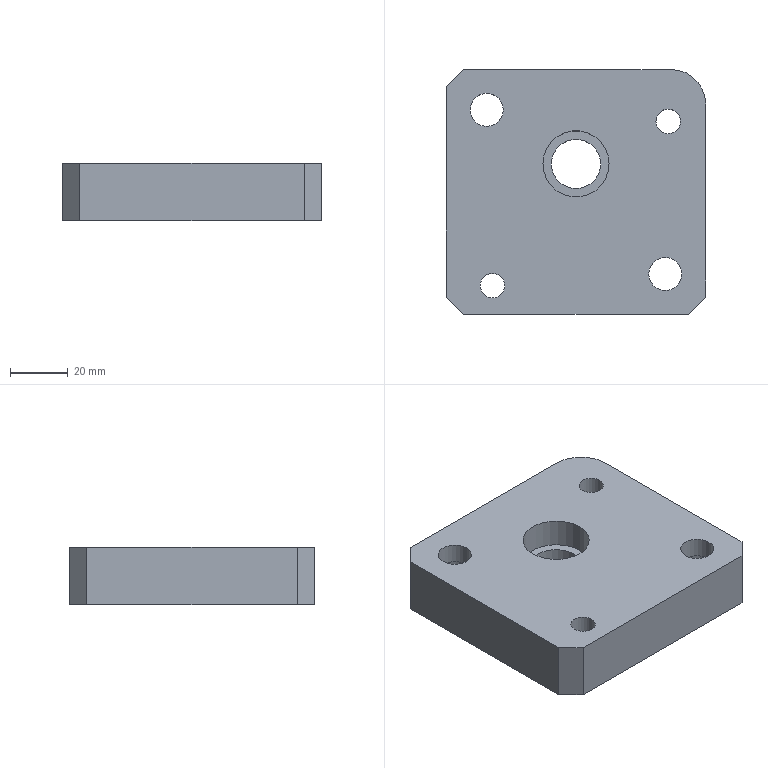Part | STEP file | lll_id3138_x_t | 1 solid | 21 faces | box 90 x 85 x 20 mm | volume 134500 mm3 | plane 12 | cylinder 9 | commonest cylinder face diameters 8.505 x2 11.509 x2 18.007 x2 17.1 x1 23 x1 24 x1
STEP:
#1=CARTESIAN_POINT('',(403.747,257.75,2.5));
#2=VERTEX_POINT('',#1);
#3=CARTESIAN_POINT('',(408.,257.75,2.5));
#4=DIRECTION('',(0.,0.,-1.));
#5=DIRECTION('',(-1.,0.,0.));
#6=AXIS2_PLACEMENT_3D('',#3,#4,#5);
#7=CIRCLE('',#6,4.253);
#8=EDGE_CURVE('',#2,#2,#7,.T.);
#9=ORIENTED_EDGE('',*,*,#8,.F.);
#10=EDGE_LOOP('',(#9));
#11=FACE_BOUND('',#10,.T.);
#12=CARTESIAN_POINT('',(415.003,318.75,2.5));
#13=VERTEX_POINT('',#12);
#14=CARTESIAN_POINT('',(406.,318.75,2.5));
#15=DIRECTION('',(0.,0.,1.));
#16=DIRECTION('',(1.,0.,0.));
#17=AXIS2_PLACEMENT_3D('',#14,#15,#16);
#18=CIRCLE('',#17,9.004);
#19=EDGE_CURVE('',#13,#13,#18,.T.);
#20=ORIENTED_EDGE('',*,*,#19,.T.);
#21=EDGE_LOOP('',(#20));
#22=FACE_BOUND('',#21,.T.);
#23=CARTESIAN_POINT('',(464.747,314.75,2.5));
#24=VERTEX_POINT('',#23);
#25=CARTESIAN_POINT('',(469.,314.75,2.5));
#26=DIRECTION('',(0.,0.,-1.));
#27=DIRECTION('',(-1.,0.,0.));
#28=AXIS2_PLACEMENT_3D('',#25,#26,#27);
#29=CIRCLE('',#28,4.253);
#30=EDGE_CURVE('',#24,#24,#29,.T.);
#31=ORIENTED_EDGE('',*,*,#30,.F.);
#32=EDGE_LOOP('',(#31));
#33=FACE_BOUND('',#32,.T.);
#34=CARTESIAN_POINT('',(470.,332.75,2.5));
#35=VERTEX_POINT('',#34);
#36=CARTESIAN_POINT('',(398.,332.75,2.5));
#37=VERTEX_POINT('',#36);
#38=CARTESIAN_POINT('',(437.,332.75,2.5));
#39=DIRECTION('',(-1.,0.,0.));
#40=VECTOR('',#39,1.);
#41=LINE('',#38,#40);
#42=EDGE_CURVE('',#35,#37,#41,.T.);
#43=ORIENTED_EDGE('',*,*,#42,.F.);
#44=CARTESIAN_POINT('',(482.,320.75,2.5));
#45=VERTEX_POINT('',#44);
#46=CARTESIAN_POINT('',(470.,320.75,2.5));
#47=DIRECTION('',(0.,0.,-1.));
#48=DIRECTION('',(-1.,0.,0.));
#49=AXIS2_PLACEMENT_3D('',#46,#47,#48);
#50=CIRCLE('',#49,12.);
#51=EDGE_CURVE('',#35,#45,#50,.T.);
#52=ORIENTED_EDGE('',*,*,#51,.T.);
#53=CARTESIAN_POINT('',(482.,253.75,2.5));
#54=VERTEX_POINT('',#53);
#55=CARTESIAN_POINT('',(482.,291.75,2.5));
#56=DIRECTION('',(0.,1.,0.));
#57=VECTOR('',#56,1.);
#58=LINE('',#55,#57);
#59=EDGE_CURVE('',#54,#45,#58,.T.);
#60=ORIENTED_EDGE('',*,*,#59,.F.);
#61=CARTESIAN_POINT('',(476.,247.75,2.5));
#62=VERTEX_POINT('',#61);
#63=CARTESIAN_POINT('',(478.5,250.25,2.5));
#64=DIRECTION('',(-0.7071,-0.7071,0.));
#65=VECTOR('',#64,1.);
#66=LINE('',#63,#65);
#67=EDGE_CURVE('',#54,#62,#66,.T.);
#68=ORIENTED_EDGE('',*,*,#67,.T.);
#69=CARTESIAN_POINT('',(398.,247.75,2.5));
#70=VERTEX_POINT('',#69);
#71=CARTESIAN_POINT('',(437.,247.75,2.5));
#72=DIRECTION('',(1.,0.,0.));
#73=VECTOR('',#72,1.);
#74=LINE('',#71,#73);
#75=EDGE_CURVE('',#70,#62,#74,.T.);
#76=ORIENTED_EDGE('',*,*,#75,.F.);
#77=CARTESIAN_POINT('',(392.,253.75,2.5));
#78=VERTEX_POINT('',#77);
#79=CARTESIAN_POINT('',(395.5,250.25,2.5));
#80=DIRECTION('',(-0.7071,0.7071,0.));
#81=VECTOR('',#80,1.);
#82=LINE('',#79,#81);
#83=EDGE_CURVE('',#70,#78,#82,.T.);
#84=ORIENTED_EDGE('',*,*,#83,.T.);
#85=CARTESIAN_POINT('',(392.,326.75,2.5));
#86=VERTEX_POINT('',#85);
#87=CARTESIAN_POINT('',(392.,291.75,2.5));
#88=DIRECTION('',(0.,-1.,0.));
#89=VECTOR('',#88,1.);
#90=LINE('',#87,#89);
#91=EDGE_CURVE('',#86,#78,#90,.T.);
#92=ORIENTED_EDGE('',*,*,#91,.F.);
#93=CARTESIAN_POINT('',(397.,331.75,2.5));
#94=DIRECTION('',(0.7071,0.7071,0.));
#95=VECTOR('',#94,1.);
#96=LINE('',#93,#95);
#97=EDGE_CURVE('',#86,#37,#96,.T.);
#98=ORIENTED_EDGE('',*,*,#97,.T.);
#99=EDGE_LOOP('',(#43,#52,#60,#68,#76,#84,#92,#98));
#100=FACE_BOUND('',#99,.T.);
#101=CARTESIAN_POINT('',(428.45,300.,2.5));
#102=VERTEX_POINT('',#101);
#103=CARTESIAN_POINT('',(437.,300.,2.5));
#104=DIRECTION('',(0.,0.,1.));
#105=DIRECTION('',(-1.,0.,0.));
#106=AXIS2_PLACEMENT_3D('',#103,#104,#105);
#107=CIRCLE('',#106,8.55);
#108=EDGE_CURVE('',#102,#102,#107,.T.);
#109=ORIENTED_EDGE('',*,*,#108,.T.);
#110=EDGE_LOOP('',(#109));
#111=FACE_BOUND('',#110,.T.);
#112=CARTESIAN_POINT('',(477.003,261.75,2.5));
#113=VERTEX_POINT('',#112);
#114=CARTESIAN_POINT('',(468.,261.75,2.5));
#115=DIRECTION('',(0.,0.,1.));
#116=DIRECTION('',(1.,0.,0.));
#117=AXIS2_PLACEMENT_3D('',#114,#115,#116);
#118=CIRCLE('',#117,9.004);
#119=EDGE_CURVE('',#113,#113,#118,.T.);
#120=ORIENTED_EDGE('',*,*,#119,.T.);
#121=EDGE_LOOP('',(#120));
#122=FACE_BOUND('',#121,.T.);
#123=CARTESIAN_POINT('',(437.,291.75,2.5));
#124=DIRECTION('',(0.,0.,-1.));
#125=DIRECTION('',(1.,0.,0.));
#126=AXIS2_PLACEMENT_3D('',#123,#124,#125);
#127=PLANE('',#126);
#128=ADVANCED_FACE('',(#11,#22,#33,#100,#111,#122),#127,.T.);
#129=CARTESIAN_POINT('',(412.252,257.75,22.5));
#130=VERTEX_POINT('',#129);
#131=CARTESIAN_POINT('',(408.,257.75,22.5));
#132=DIRECTION('',(0.,0.,1.));
#133=DIRECTION('',(1.,0.,0.));
#134=AXIS2_PLACEMENT_3D('',#131,#132,#133);
#135=CIRCLE('',#134,4.253);
#136=EDGE_CURVE('',#130,#130,#135,.T.);
#137=ORIENTED_EDGE('',*,*,#136,.F.);
#138=EDGE_LOOP('',(#137));
#139=FACE_BOUND('',#138,.T.);
#140=CARTESIAN_POINT('',(473.754,261.75,22.5));
#141=VERTEX_POINT('',#140);
#142=CARTESIAN_POINT('',(468.,261.75,22.5));
#143=DIRECTION('',(0.,0.,1.));
#144=DIRECTION('',(1.,0.,0.));
#145=AXIS2_PLACEMENT_3D('',#142,#143,#144);
#146=CIRCLE('',#145,5.755);
#147=EDGE_CURVE('',#141,#141,#146,.T.);
#148=ORIENTED_EDGE('',*,*,#147,.F.);
#149=EDGE_LOOP('',(#148));
#150=FACE_BOUND('',#149,.T.);
#151=CARTESIAN_POINT('',(411.754,318.75,22.5));
#152=VERTEX_POINT('',#151);
#153=CARTESIAN_POINT('',(406.,318.75,22.5));
#154=DIRECTION('',(0.,0.,1.));
#155=DIRECTION('',(1.,0.,0.));
#156=AXIS2_PLACEMENT_3D('',#153,#154,#155);
#157=CIRCLE('',#156,5.755);
#158=EDGE_CURVE('',#152,#152,#157,.T.);
#159=ORIENTED_EDGE('',*,*,#158,.F.);
#160=EDGE_LOOP('',(#159));
#161=FACE_BOUND('',#160,.T.);
#162=CARTESIAN_POINT('',(473.252,314.75,22.5));
#163=VERTEX_POINT('',#162);
#164=CARTESIAN_POINT('',(469.,314.75,22.5));
#165=DIRECTION('',(0.,0.,1.));
#166=DIRECTION('',(1.,0.,0.));
#167=AXIS2_PLACEMENT_3D('',#164,#165,#166);
#168=CIRCLE('',#167,4.253);
#169=EDGE_CURVE('',#163,#163,#168,.T.);
#170=ORIENTED_EDGE('',*,*,#169,.F.);
#171=EDGE_LOOP('',(#170));
#172=FACE_BOUND('',#171,.T.);
#173=CARTESIAN_POINT('',(482.,320.75,22.5));
#174=VERTEX_POINT('',#173);
#175=CARTESIAN_POINT('',(482.,253.75,22.5));
#176=VERTEX_POINT('',#175);
#177=CARTESIAN_POINT('',(482.,291.75,22.5));
#178=DIRECTION('',(0.,-1.,0.));
#179=VECTOR('',#178,1.);
#180=LINE('',#177,#179);
#181=EDGE_CURVE('',#174,#176,#180,.T.);
#182=ORIENTED_EDGE('',*,*,#181,.F.);
#183=CARTESIAN_POINT('',(470.,332.75,22.5));
#184=VERTEX_POINT('',#183);
#185=CARTESIAN_POINT('',(470.,320.75,22.5));
#186=DIRECTION('',(0.,0.,1.));
#187=DIRECTION('',(1.,0.,0.));
#188=AXIS2_PLACEMENT_3D('',#185,#186,#187);
#189=CIRCLE('',#188,12.);
#190=EDGE_CURVE('',#174,#184,#189,.T.);
#191=ORIENTED_EDGE('',*,*,#190,.T.);
#192=CARTESIAN_POINT('',(398.,332.75,22.5));
#193=VERTEX_POINT('',#192);
#194=CARTESIAN_POINT('',(437.,332.75,22.5));
#195=DIRECTION('',(1.,0.,0.));
#196=VECTOR('',#195,1.);
#197=LINE('',#194,#196);
#198=EDGE_CURVE('',#193,#184,#197,.T.);
#199=ORIENTED_EDGE('',*,*,#198,.F.);
#200=CARTESIAN_POINT('',(392.,326.75,22.5));
#201=VERTEX_POINT('',#200);
#202=CARTESIAN_POINT('',(397.,331.75,22.5));
#203=DIRECTION('',(-0.7071,-0.7071,0.));
#204=VECTOR('',#203,1.);
#205=LINE('',#202,#204);
#206=EDGE_CURVE('',#193,#201,#205,.T.);
#207=ORIENTED_EDGE('',*,*,#206,.T.);
#208=CARTESIAN_POINT('',(392.,253.75,22.5));
#209=VERTEX_POINT('',#208);
#210=CARTESIAN_POINT('',(392.,291.75,22.5));
#211=DIRECTION('',(0.,1.,0.));
#212=VECTOR('',#211,1.);
#213=LINE('',#210,#212);
#214=EDGE_CURVE('',#209,#201,#213,.T.);
#215=ORIENTED_EDGE('',*,*,#214,.F.);
#216=CARTESIAN_POINT('',(398.,247.75,22.5));
#217=VERTEX_POINT('',#216);
#218=CARTESIAN_POINT('',(395.5,250.25,22.5));
#219=DIRECTION('',(0.7071,-0.7071,0.));
#220=VECTOR('',#219,1.);
#221=LINE('',#218,#220);
#222=EDGE_CURVE('',#209,#217,#221,.T.);
#223=ORIENTED_EDGE('',*,*,#222,.T.);
#224=CARTESIAN_POINT('',(476.,247.75,22.5));
#225=VERTEX_POINT('',#224);
#226=CARTESIAN_POINT('',(437.,247.75,22.5));
#227=DIRECTION('',(-1.,0.,0.));
#228=VECTOR('',#227,1.);
#229=LINE('',#226,#228);
#230=EDGE_CURVE('',#225,#217,#229,.T.);
#231=ORIENTED_EDGE('',*,*,#230,.F.);
#232=CARTESIAN_POINT('',(478.5,250.25,22.5));
#233=DIRECTION('',(0.7071,0.7071,0.));
#234=VECTOR('',#233,1.);
#235=LINE('',#232,#234);
#236=EDGE_CURVE('',#225,#176,#235,.T.);
#237=ORIENTED_EDGE('',*,*,#236,.T.);
#238=EDGE_LOOP('',(#182,#191,#199,#207,#215,#223,#231,#237));
#239=FACE_BOUND('',#238,.T.);
#240=CARTESIAN_POINT('',(448.5,300.,22.5));
#241=VERTEX_POINT('',#240);
#242=CARTESIAN_POINT('',(437.,300.,22.5));
#243=DIRECTION('',(0.,0.,-1.));
#244=DIRECTION('',(1.,0.,0.));
#245=AXIS2_PLACEMENT_3D('',#242,#243,#244);
#246=CIRCLE('',#245,11.5);
#247=EDGE_CURVE('',#241,#241,#246,.T.);
#248=ORIENTED_EDGE('',*,*,#247,.T.);
#249=EDGE_LOOP('',(#248));
#250=FACE_BOUND('',#249,.T.);
#251=CARTESIAN_POINT('',(437.,291.75,22.5));
#252=DIRECTION('',(0.,0.,1.));
#253=DIRECTION('',(-1.,0.,0.));
#254=AXIS2_PLACEMENT_3D('',#251,#252,#253);
#255=PLANE('',#254);
#256=ADVANCED_FACE('',(#139,#150,#161,#172,#239,#250),#255,.T.);
#257=ORIENTED_EDGE('',*,*,#198,.T.);
#258=CARTESIAN_POINT('',(470.,332.75,2.5));
#259=DIRECTION('',(0.,0.,-1.));
#260=VECTOR('',#259,1.);
#261=LINE('',#258,#260);
#262=EDGE_CURVE('',#184,#35,#261,.T.);
#263=ORIENTED_EDGE('',*,*,#262,.T.);
#264=ORIENTED_EDGE('',*,*,#42,.T.);
#265=CARTESIAN_POINT('',(398.,332.75,2.5));
#266=DIRECTION('',(0.,0.,1.));
#267=VECTOR('',#266,1.);
#268=LINE('',#265,#267);
#269=EDGE_CURVE('',#37,#193,#268,.T.);
#270=ORIENTED_EDGE('',*,*,#269,.T.);
#271=EDGE_LOOP('',(#257,#263,#264,#270));
#272=FACE_OUTER_BOUND('',#271,.T.);
#273=CARTESIAN_POINT('',(437.,332.75,2.5));
#274=DIRECTION('',(0.,1.,0.));
#275=DIRECTION('',(0.,0.,-1.));
#276=AXIS2_PLACEMENT_3D('',#273,#274,#275);
#277=PLANE('',#276);
#278=ADVANCED_FACE('',(#272),#277,.T.);
#279=ORIENTED_EDGE('',*,*,#59,.T.);
#280=CARTESIAN_POINT('',(482.,320.75,2.5));
#281=DIRECTION('',(0.,0.,1.));
#282=VECTOR('',#281,1.);
#283=LINE('',#280,#282);
#284=EDGE_CURVE('',#45,#174,#283,.T.);
#285=ORIENTED_EDGE('',*,*,#284,.T.);
#286=ORIENTED_EDGE('',*,*,#181,.T.);
#287=CARTESIAN_POINT('',(482.,253.75,2.5));
#288=DIRECTION('',(0.,0.,-1.));
#289=VECTOR('',#288,1.);
#290=LINE('',#287,#289);
#291=EDGE_CURVE('',#176,#54,#290,.T.);
#292=ORIENTED_EDGE('',*,*,#291,.T.);
#293=EDGE_LOOP('',(#279,#285,#286,#292));
#294=FACE_OUTER_BOUND('',#293,.T.);
#295=CARTESIAN_POINT('',(482.,291.75,2.5));
#296=DIRECTION('',(1.,0.,0.));
#297=DIRECTION('',(0.,0.,1.));
#298=AXIS2_PLACEMENT_3D('',#295,#296,#297);
#299=PLANE('',#298);
#300=ADVANCED_FACE('',(#294),#299,.T.);
#301=ORIENTED_EDGE('',*,*,#75,.T.);
#302=CARTESIAN_POINT('',(476.,247.75,2.5));
#303=DIRECTION('',(0.,0.,1.));
#304=VECTOR('',#303,1.);
#305=LINE('',#302,#304);
#306=EDGE_CURVE('',#62,#225,#305,.T.);
#307=ORIENTED_EDGE('',*,*,#306,.T.);
#308=ORIENTED_EDGE('',*,*,#230,.T.);
#309=CARTESIAN_POINT('',(398.,247.75,2.5));
#310=DIRECTION('',(0.,0.,-1.));
#311=VECTOR('',#310,1.);
#312=LINE('',#309,#311);
#313=EDGE_CURVE('',#217,#70,#312,.T.);
#314=ORIENTED_EDGE('',*,*,#313,.T.);
#315=EDGE_LOOP('',(#301,#307,#308,#314));
#316=FACE_OUTER_BOUND('',#315,.T.);
#317=CARTESIAN_POINT('',(437.,247.75,2.5));
#318=DIRECTION('',(0.,-1.,0.));
#319=DIRECTION('',(0.,0.,1.));
#320=AXIS2_PLACEMENT_3D('',#317,#318,#319);
#321=PLANE('',#320);
#322=ADVANCED_FACE('',(#316),#321,.T.);
#323=ORIENTED_EDGE('',*,*,#214,.T.);
#324=CARTESIAN_POINT('',(392.,326.75,2.5));
#325=DIRECTION('',(0.,0.,-1.));
#326=VECTOR('',#325,1.);
#327=LINE('',#324,#326);
#328=EDGE_CURVE('',#201,#86,#327,.T.);
#329=ORIENTED_EDGE('',*,*,#328,.T.);
#330=ORIENTED_EDGE('',*,*,#91,.T.);
#331=CARTESIAN_POINT('',(392.,253.75,2.5));
#332=DIRECTION('',(0.,0.,1.));
#333=VECTOR('',#332,1.);
#334=LINE('',#331,#333);
#335=EDGE_CURVE('',#78,#209,#334,.T.);
#336=ORIENTED_EDGE('',*,*,#335,.T.);
#337=EDGE_LOOP('',(#323,#329,#330,#336));
#338=FACE_OUTER_BOUND('',#337,.T.);
#339=CARTESIAN_POINT('',(392.,291.75,2.5));
#340=DIRECTION('',(-1.,0.,0.));
#341=DIRECTION('',(0.,0.,-1.));
#342=AXIS2_PLACEMENT_3D('',#339,#340,#341);
#343=PLANE('',#342);
#344=ADVANCED_FACE('',(#338),#343,.T.);
#345=CARTESIAN_POINT('',(428.45,300.,12.5));
#346=VERTEX_POINT('',#345);
#347=CARTESIAN_POINT('',(437.,300.,12.5));
#348=DIRECTION('',(0.,0.,-1.));
#349=DIRECTION('',(-1.,0.,0.));
#350=AXIS2_PLACEMENT_3D('',#347,#348,#349);
#351=CIRCLE('',#350,8.55);
#352=EDGE_CURVE('',#346,#346,#351,.T.);
#353=ORIENTED_EDGE('',*,*,#352,.F.);
#354=EDGE_LOOP('',(#353));
#355=FACE_BOUND('',#354,.T.);
#356=ORIENTED_EDGE('',*,*,#108,.F.);
#357=EDGE_LOOP('',(#356));
#358=FACE_BOUND('',#357,.T.);
#359=CARTESIAN_POINT('',(437.,300.,125.));
#360=DIRECTION('',(0.,0.,-1.));
#361=DIRECTION('',(1.,0.,0.));
#362=AXIS2_PLACEMENT_3D('',#359,#360,#361);
#363=CYLINDRICAL_SURFACE('',#362,8.55);
#364=ADVANCED_FACE('',(#355,#358),#363,.F.);
#365=CARTESIAN_POINT('',(425.5,300.,12.5));
#366=VERTEX_POINT('',#365);
#367=CARTESIAN_POINT('',(437.,300.,12.5));
#368=DIRECTION('',(0.,0.,1.));
#369=DIRECTION('',(-1.,0.,0.));
#370=AXIS2_PLACEMENT_3D('',#367,#368,#369);
#371=CIRCLE('',#370,11.5);
#372=EDGE_CURVE('',#366,#366,#371,.T.);
#373=ORIENTED_EDGE('',*,*,#372,.F.);
#374=EDGE_LOOP('',(#373));
#375=FACE_BOUND('',#374,.T.);
#376=ORIENTED_EDGE('',*,*,#247,.F.);
#377=EDGE_LOOP('',(#376));
#378=FACE_BOUND('',#377,.T.);
#379=CARTESIAN_POINT('',(437.,300.,12.5));
#380=DIRECTION('',(0.,0.,1.));
#381=DIRECTION('',(1.,0.,0.));
#382=AXIS2_PLACEMENT_3D('',#379,#380,#381);
#383=CYLINDRICAL_SURFACE('',#382,11.5);
#384=ADVANCED_FACE('',(#375,#378),#383,.F.);
#385=ORIENTED_EDGE('',*,*,#352,.T.);
#386=EDGE_LOOP('',(#385));
#387=FACE_BOUND('',#386,.T.);
#388=ORIENTED_EDGE('',*,*,#372,.T.);
#389=EDGE_LOOP('',(#388));
#390=FACE_BOUND('',#389,.T.);
#391=CARTESIAN_POINT('',(437.,300.,12.5));
#392=DIRECTION('',(0.,0.,-1.));
#393=DIRECTION('',(-1.,0.,0.));
#394=AXIS2_PLACEMENT_3D('',#391,#392,#393);
#395=PLANE('',#394);
#396=ADVANCED_FACE('',(#387,#390),#395,.F.);
#397=ORIENTED_EDGE('',*,*,#169,.T.);
#398=EDGE_LOOP('',(#397));
#399=FACE_BOUND('',#398,.T.);
#400=ORIENTED_EDGE('',*,*,#30,.T.);
#401=EDGE_LOOP('',(#400));
#402=FACE_BOUND('',#401,.T.);
#403=CARTESIAN_POINT('',(469.,314.75,-2.5));
#404=DIRECTION('',(0.,0.,1.));
#405=DIRECTION('',(1.,0.,0.));
#406=AXIS2_PLACEMENT_3D('',#403,#404,#405);
#407=CYLINDRICAL_SURFACE('',#406,4.253);
#408=ADVANCED_FACE('',(#399,#402),#407,.F.);
#409=ORIENTED_EDGE('',*,*,#158,.T.);
#410=EDGE_LOOP('',(#409));
#411=FACE_BOUND('',#410,.T.);
#412=CARTESIAN_POINT('',(411.754,318.75,15.5));
#413=VERTEX_POINT('',#412);
#414=CARTESIAN_POINT('',(406.,318.75,15.5));
#415=DIRECTION('',(0.,0.,1.));
#416=DIRECTION('',(1.,0.,0.));
#417=AXIS2_PLACEMENT_3D('',#414,#415,#416);
#418=CIRCLE('',#417,5.755);
#419=EDGE_CURVE('',#413,#413,#418,.T.);
#420=ORIENTED_EDGE('',*,*,#419,.F.);
#421=EDGE_LOOP('',(#420));
#422=FACE_BOUND('',#421,.T.);
#423=CARTESIAN_POINT('',(406.,318.75,-2.5));
#424=DIRECTION('',(0.,0.,1.));
#425=DIRECTION('',(1.,0.,0.));
#426=AXIS2_PLACEMENT_3D('',#423,#424,#425);
#427=CYLINDRICAL_SURFACE('',#426,5.755);
#428=ADVANCED_FACE('',(#411,#422),#427,.F.);
#429=ORIENTED_EDGE('',*,*,#419,.T.);
#430=EDGE_LOOP('',(#429));
#431=FACE_BOUND('',#430,.T.);
#432=CARTESIAN_POINT('',(415.003,318.75,15.5));
#433=VERTEX_POINT('',#432);
#434=CARTESIAN_POINT('',(406.,318.75,15.5));
#435=DIRECTION('',(0.,0.,1.));
#436=DIRECTION('',(1.,0.,0.));
#437=AXIS2_PLACEMENT_3D('',#434,#435,#436);
#438=CIRCLE('',#437,9.004);
#439=EDGE_CURVE('',#433,#433,#438,.T.);
#440=ORIENTED_EDGE('',*,*,#439,.F.);
#441=EDGE_LOOP('',(#440));
#442=FACE_BOUND('',#441,.T.);
#443=CARTESIAN_POINT('',(406.,318.75,15.5));
#444=DIRECTION('',(0.,0.,1.));
#445=DIRECTION('',(1.,0.,0.));
#446=AXIS2_PLACEMENT_3D('',#443,#444,#445);
#447=PLANE('',#446);
#448=ADVANCED_FACE('',(#431,#442),#447,.F.);
#449=ORIENTED_EDGE('',*,*,#439,.T.);
#450=EDGE_LOOP('',(#449));
#451=FACE_BOUND('',#450,.T.);
#452=ORIENTED_EDGE('',*,*,#19,.F.);
#453=EDGE_LOOP('',(#452));
#454=FACE_BOUND('',#453,.T.);
#455=CARTESIAN_POINT('',(406.,318.75,2.5));
#456=DIRECTION('',(0.,0.,1.));
#457=DIRECTION('',(1.,0.,0.));
#458=AXIS2_PLACEMENT_3D('',#455,#456,#457);
#459=CYLINDRICAL_SURFACE('',#458,9.004);
#460=ADVANCED_FACE('',(#451,#454),#459,.F.);
#461=ORIENTED_EDGE('',*,*,#147,.T.);
#462=EDGE_LOOP('',(#461));
#463=FACE_BOUND('',#462,.T.);
#464=CARTESIAN_POINT('',(473.754,261.75,15.5));
#465=VERTEX_POINT('',#464);
#466=CARTESIAN_POINT('',(468.,261.75,15.5));
#467=DIRECTION('',(0.,0.,1.));
#468=DIRECTION('',(1.,0.,0.));
#469=AXIS2_PLACEMENT_3D('',#466,#467,#468);
#470=CIRCLE('',#469,5.755);
#471=EDGE_CURVE('',#465,#465,#470,.T.);
#472=ORIENTED_EDGE('',*,*,#471,.F.);
#473=EDGE_LOOP('',(#472));
#474=FACE_BOUND('',#473,.T.);
#475=CARTESIAN_POINT('',(468.,261.75,-2.5));
#476=DIRECTION('',(0.,0.,1.));
#477=DIRECTION('',(1.,0.,0.));
#478=AXIS2_PLACEMENT_3D('',#475,#476,#477);
#479=CYLINDRICAL_SURFACE('',#478,5.755);
#480=ADVANCED_FACE('',(#463,#474),#479,.F.);
#481=ORIENTED_EDGE('',*,*,#471,.T.);
#482=EDGE_LOOP('',(#481));
#483=FACE_BOUND('',#482,.T.);
#484=CARTESIAN_POINT('',(477.003,261.75,15.5));
#485=VERTEX_POINT('',#484);
#486=CARTESIAN_POINT('',(468.,261.75,15.5));
#487=DIRECTION('',(0.,0.,1.));
#488=DIRECTION('',(1.,0.,0.));
#489=AXIS2_PLACEMENT_3D('',#486,#487,#488);
#490=CIRCLE('',#489,9.004);
#491=EDGE_CURVE('',#485,#485,#490,.T.);
#492=ORIENTED_EDGE('',*,*,#491,.F.);
#493=EDGE_LOOP('',(#492));
#494=FACE_BOUND('',#493,.T.);
#495=CARTESIAN_POINT('',(468.,261.75,15.5));
#496=DIRECTION('',(0.,0.,1.));
#497=DIRECTION('',(1.,0.,0.));
#498=AXIS2_PLACEMENT_3D('',#495,#496,#497);
#499=PLANE('',#498);
#500=ADVANCED_FACE('',(#483,#494),#499,.F.);
#501=ORIENTED_EDGE('',*,*,#491,.T.);
#502=EDGE_LOOP('',(#501));
#503=FACE_BOUND('',#502,.T.);
#504=ORIENTED_EDGE('',*,*,#119,.F.);
#505=EDGE_LOOP('',(#504));
#506=FACE_BOUND('',#505,.T.);
#507=CARTESIAN_POINT('',(468.,261.75,2.5));
#508=DIRECTION('',(0.,0.,1.));
#509=DIRECTION('',(1.,0.,0.));
#510=AXIS2_PLACEMENT_3D('',#507,#508,#509);
#511=CYLINDRICAL_SURFACE('',#510,9.004);
#512=ADVANCED_FACE('',(#503,#506),#511,.F.);
#513=ORIENTED_EDGE('',*,*,#8,.T.);
#514=EDGE_LOOP('',(#513));
#515=FACE_BOUND('',#514,.T.);
#516=ORIENTED_EDGE('',*,*,#136,.T.);
#517=EDGE_LOOP('',(#516));
#518=FACE_BOUND('',#517,.T.);
#519=CARTESIAN_POINT('',(408.,257.75,-2.5));
#520=DIRECTION('',(0.,0.,1.));
#521=DIRECTION('',(1.,0.,0.));
#522=AXIS2_PLACEMENT_3D('',#519,#520,#521);
#523=CYLINDRICAL_SURFACE('',#522,4.253);
#524=ADVANCED_FACE('',(#515,#518),#523,.F.);
#525=ORIENTED_EDGE('',*,*,#97,.F.);
#526=ORIENTED_EDGE('',*,*,#328,.F.);
#527=ORIENTED_EDGE('',*,*,#206,.F.);
#528=ORIENTED_EDGE('',*,*,#269,.F.);
#529=EDGE_LOOP('',(#525,#526,#527,#528));
#530=FACE_OUTER_BOUND('',#529,.T.);
#531=CARTESIAN_POINT('',(398.,332.75,2.5));
#532=DIRECTION('',(0.7071,-0.7071,0.));
#533=DIRECTION('',(0.,0.,-1.));
#534=AXIS2_PLACEMENT_3D('',#531,#532,#533);
#535=PLANE('',#534);
#536=ADVANCED_FACE('',(#530),#535,.F.);
#537=ORIENTED_EDGE('',*,*,#67,.F.);
#538=ORIENTED_EDGE('',*,*,#291,.F.);
#539=ORIENTED_EDGE('',*,*,#236,.F.);
#540=ORIENTED_EDGE('',*,*,#306,.F.);
#541=EDGE_LOOP('',(#537,#538,#539,#540));
#542=FACE_OUTER_BOUND('',#541,.T.);
#543=CARTESIAN_POINT('',(476.,247.75,2.5));
#544=DIRECTION('',(-0.7071,0.7071,0.));
#545=DIRECTION('',(0.,0.,-1.));
#546=AXIS2_PLACEMENT_3D('',#543,#544,#545);
#547=PLANE('',#546);
#548=ADVANCED_FACE('',(#542),#547,.F.);
#549=ORIENTED_EDGE('',*,*,#83,.F.);
#550=ORIENTED_EDGE('',*,*,#313,.F.);
#551=ORIENTED_EDGE('',*,*,#222,.F.);
#552=ORIENTED_EDGE('',*,*,#335,.F.);
#553=EDGE_LOOP('',(#549,#550,#551,#552));
#554=FACE_OUTER_BOUND('',#553,.T.);
#555=CARTESIAN_POINT('',(392.,253.75,2.5));
#556=DIRECTION('',(0.7071,0.7071,0.));
#557=DIRECTION('',(0.,0.,-1.));
#558=AXIS2_PLACEMENT_3D('',#555,#556,#557);
#559=PLANE('',#558);
#560=ADVANCED_FACE('',(#554),#559,.F.);
#561=ORIENTED_EDGE('',*,*,#190,.F.);
#562=ORIENTED_EDGE('',*,*,#284,.F.);
#563=ORIENTED_EDGE('',*,*,#51,.F.);
#564=ORIENTED_EDGE('',*,*,#262,.F.);
#565=EDGE_LOOP('',(#561,#562,#563,#564));
#566=FACE_OUTER_BOUND('',#565,.T.);
#567=CARTESIAN_POINT('',(470.,320.75,2.5));
#568=DIRECTION('',(0.,0.,-1.));
#569=DIRECTION('',(1.,0.,0.));
#570=AXIS2_PLACEMENT_3D('',#567,#568,#569);
#571=CYLINDRICAL_SURFACE('',#570,12.);
#572=ADVANCED_FACE('',(#566),#571,.T.);
#573=CLOSED_SHELL('',(#128,#256,#278,#300,#322,#344,#364,#384,#396,#408,#428,#448,#460,#480,#500,#512,#524,#536,#548,#560,#572));
#574=MANIFOLD_SOLID_BREP('',#573);
#575=(LENGTH_UNIT()NAMED_UNIT(*)SI_UNIT(.MILLI.,.METRE.));
#576=UNCERTAINTY_MEASURE_WITH_UNIT(LENGTH_MEASURE(0.00002),#575,'','');
#577=(NAMED_UNIT(*)PLANE_ANGLE_UNIT()SI_UNIT($,.RADIAN.));
#578=PLANE_ANGLE_MEASURE_WITH_UNIT(PLANE_ANGLE_MEASURE(0.01745),#577);
#579=DIMENSIONAL_EXPONENTS(0.,0.,0.,0.,0.,0.,0.);
#580=(CONVERSION_BASED_UNIT('DEGREE',#578)NAMED_UNIT(#579)PLANE_ANGLE_UNIT());
#581=(NAMED_UNIT(*)SI_UNIT($,.STERADIAN.)SOLID_ANGLE_UNIT());
#582=(GEOMETRIC_REPRESENTATION_CONTEXT(3)GLOBAL_UNCERTAINTY_ASSIGNED_CONTEXT((#576))GLOBAL_UNIT_ASSIGNED_CONTEXT((#575,#580,#581))REPRESENTATION_CONTEXT('',''));
#583=ADVANCED_BREP_SHAPE_REPRESENTATION('',(#574),#582);